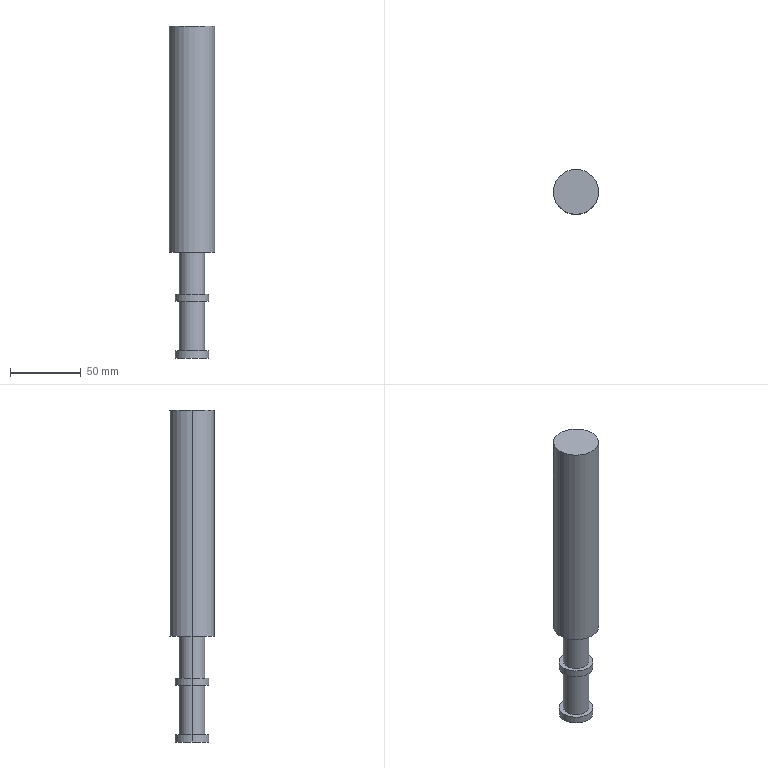Part | SolidWorks | features ICE 4, LPattern 1 | 1 solid | 16 faces | box 32 x 32 x 235 mm | volume 149708 mm3 | cylinder 10 | plane 6 | commonest cylinder face diameters 18 x4 23.904 x4 32 x2
STEP:
#1=CARTESIAN_POINT('',(-28.201,5.869,-90.));
#2=VERTEX_POINT('',#1);
#3=CARTESIAN_POINT('',(-10.201,5.869,-90.));
#4=VERTEX_POINT('',#3);
#5=CARTESIAN_POINT('',(-19.201,5.869,-90.));
#6=DIRECTION('',(0.,0.,-1.));
#7=DIRECTION('',(-1.,0.,0.));
#8=AXIS2_PLACEMENT_3D('',#5,#6,#7);
#9=CIRCLE('',#8,9.);
#10=EDGE_CURVE('',#2,#4,#9,.T.);
#11=ORIENTED_EDGE('',*,*,#10,.F.);
#12=CARTESIAN_POINT('',(-28.201,5.869,-60.));
#13=VERTEX_POINT('',#12);
#14=CARTESIAN_POINT('',(-28.201,5.869,-130.));
#15=DIRECTION('',(0.,0.,1.));
#16=VECTOR('',#15,1000.);
#17=LINE('',#14,#16);
#18=EDGE_CURVE('',#2,#13,#17,.T.);
#19=ORIENTED_EDGE('',*,*,#18,.T.);
#20=CARTESIAN_POINT('',(-10.201,5.869,-60.));
#21=VERTEX_POINT('',#20);
#22=CARTESIAN_POINT('',(-19.201,5.869,-60.));
#23=DIRECTION('',(0.,0.,-1.));
#24=DIRECTION('',(-1.,0.,0.));
#25=AXIS2_PLACEMENT_3D('',#22,#23,#24);
#26=CIRCLE('',#25,9.);
#27=EDGE_CURVE('',#13,#21,#26,.T.);
#28=ORIENTED_EDGE('',*,*,#27,.T.);
#29=CARTESIAN_POINT('',(-10.201,5.869,-130.));
#30=DIRECTION('',(0.,0.,1.));
#31=VECTOR('',#30,1000.);
#32=LINE('',#29,#31);
#33=EDGE_CURVE('',#4,#21,#32,.T.);
#34=ORIENTED_EDGE('',*,*,#33,.F.);
#35=EDGE_LOOP('',(#11,#19,#28,#34));
#36=FACE_OUTER_BOUND('',#35,.T.);
#37=CARTESIAN_POINT('',(-19.201,5.869,-130.));
#38=DIRECTION('',(0.,0.,1.));
#39=DIRECTION('',(1.,0.,0.));
#40=AXIS2_PLACEMENT_3D('',#37,#38,#39);
#41=CYLINDRICAL_SURFACE('',#40,9.);
#42=ADVANCED_FACE('',(#36),#41,.T.);
#43=CARTESIAN_POINT('',(-3.201,5.869,-60.));
#44=VERTEX_POINT('',#43);
#45=CARTESIAN_POINT('',(-35.201,5.869,-60.));
#46=VERTEX_POINT('',#45);
#47=CARTESIAN_POINT('',(-19.201,5.869,-60.));
#48=DIRECTION('',(0.,0.,1.));
#49=DIRECTION('',(1.,0.,0.));
#50=AXIS2_PLACEMENT_3D('',#47,#48,#49);
#51=CIRCLE('',#50,16.);
#52=EDGE_CURVE('',#44,#46,#51,.T.);
#53=ORIENTED_EDGE('',*,*,#52,.T.);
#54=CARTESIAN_POINT('',(-35.201,5.869,100.));
#55=VERTEX_POINT('',#54);
#56=CARTESIAN_POINT('',(-35.201,5.869,-60.));
#57=DIRECTION('',(0.,0.,1.));
#58=VECTOR('',#57,1000.);
#59=LINE('',#56,#58);
#60=EDGE_CURVE('',#46,#55,#59,.T.);
#61=ORIENTED_EDGE('',*,*,#60,.T.);
#62=CARTESIAN_POINT('',(-3.201,5.869,100.));
#63=VERTEX_POINT('',#62);
#64=CARTESIAN_POINT('',(-19.201,5.869,100.));
#65=DIRECTION('',(0.,0.,1.));
#66=DIRECTION('',(1.,0.,0.));
#67=AXIS2_PLACEMENT_3D('',#64,#65,#66);
#68=CIRCLE('',#67,16.);
#69=EDGE_CURVE('',#63,#55,#68,.T.);
#70=ORIENTED_EDGE('',*,*,#69,.F.);
#71=CARTESIAN_POINT('',(-3.201,5.869,-60.));
#72=DIRECTION('',(0.,0.,1.));
#73=VECTOR('',#72,1000.);
#74=LINE('',#71,#73);
#75=EDGE_CURVE('',#44,#63,#74,.T.);
#76=ORIENTED_EDGE('',*,*,#75,.F.);
#77=EDGE_LOOP('',(#53,#61,#70,#76));
#78=FACE_OUTER_BOUND('',#77,.T.);
#79=CARTESIAN_POINT('',(-19.201,5.869,-60.));
#80=DIRECTION('',(0.,0.,1.));
#81=DIRECTION('',(1.,0.,0.));
#82=AXIS2_PLACEMENT_3D('',#79,#80,#81);
#83=CYLINDRICAL_SURFACE('',#82,16.);
#84=ADVANCED_FACE('',(#78),#83,.T.);
#85=CARTESIAN_POINT('',(-31.153,5.869,-95.));
#86=VERTEX_POINT('',#85);
#87=CARTESIAN_POINT('',(-7.249,5.869,-95.));
#88=VERTEX_POINT('',#87);
#89=CARTESIAN_POINT('',(-19.201,5.869,-95.));
#90=DIRECTION('',(0.,0.,-1.));
#91=DIRECTION('',(-1.,0.,0.));
#92=AXIS2_PLACEMENT_3D('',#89,#90,#91);
#93=CIRCLE('',#92,11.952);
#94=EDGE_CURVE('',#86,#88,#93,.T.);
#95=ORIENTED_EDGE('',*,*,#94,.F.);
#96=CARTESIAN_POINT('',(-31.153,5.869,-90.));
#97=VERTEX_POINT('',#96);
#98=CARTESIAN_POINT('',(-31.153,5.869,-95.));
#99=DIRECTION('',(0.,0.,1.));
#100=VECTOR('',#99,1000.);
#101=LINE('',#98,#100);
#102=EDGE_CURVE('',#86,#97,#101,.T.);
#103=ORIENTED_EDGE('',*,*,#102,.T.);
#104=CARTESIAN_POINT('',(-7.249,5.869,-90.));
#105=VERTEX_POINT('',#104);
#106=CARTESIAN_POINT('',(-19.201,5.869,-90.));
#107=DIRECTION('',(0.,0.,-1.));
#108=DIRECTION('',(-1.,0.,0.));
#109=AXIS2_PLACEMENT_3D('',#106,#107,#108);
#110=CIRCLE('',#109,11.952);
#111=EDGE_CURVE('',#97,#105,#110,.T.);
#112=ORIENTED_EDGE('',*,*,#111,.T.);
#113=CARTESIAN_POINT('',(-7.249,5.869,-95.));
#114=DIRECTION('',(0.,0.,1.));
#115=VECTOR('',#114,1000.);
#116=LINE('',#113,#115);
#117=EDGE_CURVE('',#88,#105,#116,.T.);
#118=ORIENTED_EDGE('',*,*,#117,.F.);
#119=EDGE_LOOP('',(#95,#103,#112,#118));
#120=FACE_OUTER_BOUND('',#119,.T.);
#121=CARTESIAN_POINT('',(-19.201,5.869,-95.));
#122=DIRECTION('',(0.,0.,1.));
#123=DIRECTION('',(1.,0.,0.));
#124=AXIS2_PLACEMENT_3D('',#121,#122,#123);
#125=CYLINDRICAL_SURFACE('',#124,11.952);
#126=ADVANCED_FACE('',(#120),#125,.T.);
#127=CARTESIAN_POINT('',(-31.153,5.869,-135.));
#128=VERTEX_POINT('',#127);
#129=CARTESIAN_POINT('',(-7.249,5.869,-135.));
#130=VERTEX_POINT('',#129);
#131=CARTESIAN_POINT('',(-19.201,5.869,-135.));
#132=DIRECTION('',(0.,0.,-1.));
#133=DIRECTION('',(-1.,0.,0.));
#134=AXIS2_PLACEMENT_3D('',#131,#132,#133);
#135=CIRCLE('',#134,11.952);
#136=EDGE_CURVE('',#128,#130,#135,.T.);
#137=ORIENTED_EDGE('',*,*,#136,.F.);
#138=CARTESIAN_POINT('',(-31.153,5.869,-130.));
#139=VERTEX_POINT('',#138);
#140=CARTESIAN_POINT('',(-31.153,5.869,-135.));
#141=DIRECTION('',(0.,0.,1.));
#142=VECTOR('',#141,1000.);
#143=LINE('',#140,#142);
#144=EDGE_CURVE('',#128,#139,#143,.T.);
#145=ORIENTED_EDGE('',*,*,#144,.T.);
#146=CARTESIAN_POINT('',(-7.249,5.869,-130.));
#147=VERTEX_POINT('',#146);
#148=CARTESIAN_POINT('',(-19.201,5.869,-130.));
#149=DIRECTION('',(0.,0.,-1.));
#150=DIRECTION('',(-1.,0.,0.));
#151=AXIS2_PLACEMENT_3D('',#148,#149,#150);
#152=CIRCLE('',#151,11.952);
#153=EDGE_CURVE('',#139,#147,#152,.T.);
#154=ORIENTED_EDGE('',*,*,#153,.T.);
#155=CARTESIAN_POINT('',(-7.249,5.869,-135.));
#156=DIRECTION('',(0.,0.,1.));
#157=VECTOR('',#156,1000.);
#158=LINE('',#155,#157);
#159=EDGE_CURVE('',#130,#147,#158,.T.);
#160=ORIENTED_EDGE('',*,*,#159,.F.);
#161=EDGE_LOOP('',(#137,#145,#154,#160));
#162=FACE_OUTER_BOUND('',#161,.T.);
#163=CARTESIAN_POINT('',(-19.201,5.869,-135.));
#164=DIRECTION('',(0.,0.,1.));
#165=DIRECTION('',(1.,0.,0.));
#166=AXIS2_PLACEMENT_3D('',#163,#164,#165);
#167=CYLINDRICAL_SURFACE('',#166,11.952);
#168=ADVANCED_FACE('',(#162),#167,.T.);
#169=CARTESIAN_POINT('',(-28.201,5.869,-130.));
#170=VERTEX_POINT('',#169);
#171=CARTESIAN_POINT('',(-10.201,5.869,-130.));
#172=VERTEX_POINT('',#171);
#173=CARTESIAN_POINT('',(-19.201,5.869,-130.));
#174=DIRECTION('',(0.,0.,-1.));
#175=DIRECTION('',(-1.,0.,0.));
#176=AXIS2_PLACEMENT_3D('',#173,#174,#175);
#177=CIRCLE('',#176,9.);
#178=EDGE_CURVE('',#170,#172,#177,.T.);
#179=ORIENTED_EDGE('',*,*,#178,.F.);
#180=CARTESIAN_POINT('',(-28.201,5.869,-95.));
#181=VERTEX_POINT('',#180);
#182=CARTESIAN_POINT('',(-28.201,5.869,-130.));
#183=DIRECTION('',(0.,0.,1.));
#184=VECTOR('',#183,1000.);
#185=LINE('',#182,#184);
#186=EDGE_CURVE('',#170,#181,#185,.T.);
#187=ORIENTED_EDGE('',*,*,#186,.T.);
#188=CARTESIAN_POINT('',(-10.201,5.869,-95.));
#189=VERTEX_POINT('',#188);
#190=CARTESIAN_POINT('',(-19.201,5.869,-95.));
#191=DIRECTION('',(0.,0.,-1.));
#192=DIRECTION('',(-1.,0.,0.));
#193=AXIS2_PLACEMENT_3D('',#190,#191,#192);
#194=CIRCLE('',#193,9.);
#195=EDGE_CURVE('',#181,#189,#194,.T.);
#196=ORIENTED_EDGE('',*,*,#195,.T.);
#197=CARTESIAN_POINT('',(-10.201,5.869,-130.));
#198=DIRECTION('',(0.,0.,1.));
#199=VECTOR('',#198,1000.);
#200=LINE('',#197,#199);
#201=EDGE_CURVE('',#172,#189,#200,.T.);
#202=ORIENTED_EDGE('',*,*,#201,.F.);
#203=EDGE_LOOP('',(#179,#187,#196,#202));
#204=FACE_OUTER_BOUND('',#203,.T.);
#205=CARTESIAN_POINT('',(-19.201,5.869,-130.));
#206=DIRECTION('',(0.,0.,1.));
#207=DIRECTION('',(1.,0.,0.));
#208=AXIS2_PLACEMENT_3D('',#205,#206,#207);
#209=CYLINDRICAL_SURFACE('',#208,9.);
#210=ADVANCED_FACE('',(#204),#209,.T.);
#211=ORIENTED_EDGE('',*,*,#186,.F.);
#212=CARTESIAN_POINT('',(-19.201,5.869,-130.));
#213=DIRECTION('',(0.,0.,-1.));
#214=DIRECTION('',(-1.,0.,0.));
#215=AXIS2_PLACEMENT_3D('',#212,#213,#214);
#216=CIRCLE('',#215,9.);
#217=EDGE_CURVE('',#172,#170,#216,.T.);
#218=ORIENTED_EDGE('',*,*,#217,.F.);
#219=ORIENTED_EDGE('',*,*,#201,.T.);
#220=CARTESIAN_POINT('',(-19.201,5.869,-95.));
#221=DIRECTION('',(0.,0.,-1.));
#222=DIRECTION('',(-1.,0.,0.));
#223=AXIS2_PLACEMENT_3D('',#220,#221,#222);
#224=CIRCLE('',#223,9.);
#225=EDGE_CURVE('',#189,#181,#224,.T.);
#226=ORIENTED_EDGE('',*,*,#225,.T.);
#227=EDGE_LOOP('',(#211,#218,#219,#226));
#228=FACE_OUTER_BOUND('',#227,.T.);
#229=CARTESIAN_POINT('',(-19.201,5.869,-130.));
#230=DIRECTION('',(0.,0.,1.));
#231=DIRECTION('',(1.,0.,0.));
#232=AXIS2_PLACEMENT_3D('',#229,#230,#231);
#233=CYLINDRICAL_SURFACE('',#232,9.);
#234=ADVANCED_FACE('',(#228),#233,.T.);
#235=ORIENTED_EDGE('',*,*,#144,.F.);
#236=CARTESIAN_POINT('',(-19.201,5.869,-135.));
#237=DIRECTION('',(0.,0.,-1.));
#238=DIRECTION('',(-1.,0.,0.));
#239=AXIS2_PLACEMENT_3D('',#236,#237,#238);
#240=CIRCLE('',#239,11.952);
#241=EDGE_CURVE('',#130,#128,#240,.T.);
#242=ORIENTED_EDGE('',*,*,#241,.F.);
#243=ORIENTED_EDGE('',*,*,#159,.T.);
#244=CARTESIAN_POINT('',(-19.201,5.869,-130.));
#245=DIRECTION('',(0.,0.,-1.));
#246=DIRECTION('',(-1.,0.,0.));
#247=AXIS2_PLACEMENT_3D('',#244,#245,#246);
#248=CIRCLE('',#247,11.952);
#249=EDGE_CURVE('',#147,#139,#248,.T.);
#250=ORIENTED_EDGE('',*,*,#249,.T.);
#251=EDGE_LOOP('',(#235,#242,#243,#250));
#252=FACE_OUTER_BOUND('',#251,.T.);
#253=CARTESIAN_POINT('',(-19.201,5.869,-135.));
#254=DIRECTION('',(0.,0.,1.));
#255=DIRECTION('',(1.,0.,0.));
#256=AXIS2_PLACEMENT_3D('',#253,#254,#255);
#257=CYLINDRICAL_SURFACE('',#256,11.952);
#258=ADVANCED_FACE('',(#252),#257,.T.);
#259=ORIENTED_EDGE('',*,*,#241,.T.);
#260=ORIENTED_EDGE('',*,*,#136,.T.);
#261=EDGE_LOOP('',(#259,#260));
#262=FACE_OUTER_BOUND('',#261,.T.);
#263=CARTESIAN_POINT('',(-19.201,5.869,-135.));
#264=DIRECTION('',(0.,0.,-1.));
#265=DIRECTION('',(-1.,0.,0.));
#266=AXIS2_PLACEMENT_3D('',#263,#264,#265);
#267=PLANE('',#266);
#268=ADVANCED_FACE('',(#262),#267,.T.);
#269=ORIENTED_EDGE('',*,*,#217,.T.);
#270=ORIENTED_EDGE('',*,*,#178,.T.);
#271=EDGE_LOOP('',(#269,#270));
#272=FACE_BOUND('',#271,.T.);
#273=ORIENTED_EDGE('',*,*,#249,.F.);
#274=ORIENTED_EDGE('',*,*,#153,.F.);
#275=EDGE_LOOP('',(#273,#274));
#276=FACE_OUTER_BOUND('',#275,.T.);
#277=CARTESIAN_POINT('',(-19.201,5.869,-130.));
#278=DIRECTION('',(0.,0.,-1.));
#279=DIRECTION('',(-1.,0.,0.));
#280=AXIS2_PLACEMENT_3D('',#277,#278,#279);
#281=PLANE('',#280);
#282=ADVANCED_FACE('',(#272,#276),#281,.F.);
#283=ORIENTED_EDGE('',*,*,#102,.F.);
#284=CARTESIAN_POINT('',(-19.201,5.869,-95.));
#285=DIRECTION('',(0.,0.,-1.));
#286=DIRECTION('',(-1.,0.,0.));
#287=AXIS2_PLACEMENT_3D('',#284,#285,#286);
#288=CIRCLE('',#287,11.952);
#289=EDGE_CURVE('',#88,#86,#288,.T.);
#290=ORIENTED_EDGE('',*,*,#289,.F.);
#291=ORIENTED_EDGE('',*,*,#117,.T.);
#292=CARTESIAN_POINT('',(-19.201,5.869,-90.));
#293=DIRECTION('',(0.,0.,-1.));
#294=DIRECTION('',(-1.,0.,0.));
#295=AXIS2_PLACEMENT_3D('',#292,#293,#294);
#296=CIRCLE('',#295,11.952);
#297=EDGE_CURVE('',#105,#97,#296,.T.);
#298=ORIENTED_EDGE('',*,*,#297,.T.);
#299=EDGE_LOOP('',(#283,#290,#291,#298));
#300=FACE_OUTER_BOUND('',#299,.T.);
#301=CARTESIAN_POINT('',(-19.201,5.869,-95.));
#302=DIRECTION('',(0.,0.,1.));
#303=DIRECTION('',(1.,0.,0.));
#304=AXIS2_PLACEMENT_3D('',#301,#302,#303);
#305=CYLINDRICAL_SURFACE('',#304,11.952);
#306=ADVANCED_FACE('',(#300),#305,.T.);
#307=ORIENTED_EDGE('',*,*,#225,.F.);
#308=ORIENTED_EDGE('',*,*,#195,.F.);
#309=EDGE_LOOP('',(#307,#308));
#310=FACE_BOUND('',#309,.T.);
#311=ORIENTED_EDGE('',*,*,#289,.T.);
#312=ORIENTED_EDGE('',*,*,#94,.T.);
#313=EDGE_LOOP('',(#311,#312));
#314=FACE_OUTER_BOUND('',#313,.T.);
#315=CARTESIAN_POINT('',(-19.201,5.869,-95.));
#316=DIRECTION('',(0.,0.,-1.));
#317=DIRECTION('',(-1.,0.,0.));
#318=AXIS2_PLACEMENT_3D('',#315,#316,#317);
#319=PLANE('',#318);
#320=ADVANCED_FACE('',(#310,#314),#319,.T.);
#321=CARTESIAN_POINT('',(-19.201,5.869,-90.));
#322=DIRECTION('',(0.,0.,-1.));
#323=DIRECTION('',(-1.,0.,0.));
#324=AXIS2_PLACEMENT_3D('',#321,#322,#323);
#325=CIRCLE('',#324,9.);
#326=EDGE_CURVE('',#4,#2,#325,.T.);
#327=ORIENTED_EDGE('',*,*,#326,.T.);
#328=ORIENTED_EDGE('',*,*,#10,.T.);
#329=EDGE_LOOP('',(#327,#328));
#330=FACE_BOUND('',#329,.T.);
#331=ORIENTED_EDGE('',*,*,#297,.F.);
#332=ORIENTED_EDGE('',*,*,#111,.F.);
#333=EDGE_LOOP('',(#331,#332));
#334=FACE_OUTER_BOUND('',#333,.T.);
#335=CARTESIAN_POINT('',(-19.201,5.869,-90.));
#336=DIRECTION('',(0.,0.,-1.));
#337=DIRECTION('',(-1.,0.,0.));
#338=AXIS2_PLACEMENT_3D('',#335,#336,#337);
#339=PLANE('',#338);
#340=ADVANCED_FACE('',(#330,#334),#339,.F.);
#341=ORIENTED_EDGE('',*,*,#69,.T.);
#342=CARTESIAN_POINT('',(-19.201,5.869,100.));
#343=DIRECTION('',(0.,0.,1.));
#344=DIRECTION('',(1.,0.,0.));
#345=AXIS2_PLACEMENT_3D('',#342,#343,#344);
#346=CIRCLE('',#345,16.);
#347=EDGE_CURVE('',#55,#63,#346,.T.);
#348=ORIENTED_EDGE('',*,*,#347,.T.);
#349=EDGE_LOOP('',(#341,#348));
#350=FACE_OUTER_BOUND('',#349,.T.);
#351=CARTESIAN_POINT('',(-19.201,5.869,100.));
#352=DIRECTION('',(0.,0.,1.));
#353=DIRECTION('',(1.,0.,0.));
#354=AXIS2_PLACEMENT_3D('',#351,#352,#353);
#355=PLANE('',#354);
#356=ADVANCED_FACE('',(#350),#355,.T.);
#357=ORIENTED_EDGE('',*,*,#60,.F.);
#358=CARTESIAN_POINT('',(-19.201,5.869,-60.));
#359=DIRECTION('',(0.,0.,1.));
#360=DIRECTION('',(1.,0.,0.));
#361=AXIS2_PLACEMENT_3D('',#358,#359,#360);
#362=CIRCLE('',#361,16.);
#363=EDGE_CURVE('',#46,#44,#362,.T.);
#364=ORIENTED_EDGE('',*,*,#363,.T.);
#365=ORIENTED_EDGE('',*,*,#75,.T.);
#366=ORIENTED_EDGE('',*,*,#347,.F.);
#367=EDGE_LOOP('',(#357,#364,#365,#366));
#368=FACE_OUTER_BOUND('',#367,.T.);
#369=CARTESIAN_POINT('',(-19.201,5.869,-60.));
#370=DIRECTION('',(0.,0.,1.));
#371=DIRECTION('',(1.,0.,0.));
#372=AXIS2_PLACEMENT_3D('',#369,#370,#371);
#373=CYLINDRICAL_SURFACE('',#372,16.);
#374=ADVANCED_FACE('',(#368),#373,.T.);
#375=CARTESIAN_POINT('',(-19.201,5.869,-60.));
#376=DIRECTION('',(0.,0.,-1.));
#377=DIRECTION('',(-1.,0.,0.));
#378=AXIS2_PLACEMENT_3D('',#375,#376,#377);
#379=CIRCLE('',#378,9.);
#380=EDGE_CURVE('',#21,#13,#379,.T.);
#381=ORIENTED_EDGE('',*,*,#380,.F.);
#382=ORIENTED_EDGE('',*,*,#27,.F.);
#383=EDGE_LOOP('',(#381,#382));
#384=FACE_BOUND('',#383,.T.);
#385=ORIENTED_EDGE('',*,*,#52,.F.);
#386=ORIENTED_EDGE('',*,*,#363,.F.);
#387=EDGE_LOOP('',(#385,#386));
#388=FACE_OUTER_BOUND('',#387,.T.);
#389=CARTESIAN_POINT('',(-19.201,5.869,-60.));
#390=DIRECTION('',(0.,0.,1.));
#391=DIRECTION('',(1.,0.,0.));
#392=AXIS2_PLACEMENT_3D('',#389,#390,#391);
#393=PLANE('',#392);
#394=ADVANCED_FACE('',(#384,#388),#393,.F.);
#395=ORIENTED_EDGE('',*,*,#18,.F.);
#396=ORIENTED_EDGE('',*,*,#326,.F.);
#397=ORIENTED_EDGE('',*,*,#33,.T.);
#398=ORIENTED_EDGE('',*,*,#380,.T.);
#399=EDGE_LOOP('',(#395,#396,#397,#398));
#400=FACE_OUTER_BOUND('',#399,.T.);
#401=CARTESIAN_POINT('',(-19.201,5.869,-130.));
#402=DIRECTION('',(0.,0.,1.));
#403=DIRECTION('',(1.,0.,0.));
#404=AXIS2_PLACEMENT_3D('',#401,#402,#403);
#405=CYLINDRICAL_SURFACE('',#404,9.);
#406=ADVANCED_FACE('',(#400),#405,.T.);
#407=CLOSED_SHELL('',(#42,#84,#126,#168,#210,#234,#258,#268,#282,#306,#320,#340,#356,#374,#394,#406));
#408=MANIFOLD_SOLID_BREP('',#407);
#409=CARTESIAN_POINT('',(0.,0.,0.));
#410=DIRECTION('',(0.,0.,1.));
#411=DIRECTION('',(1.,0.,0.));
#412=AXIS2_PLACEMENT_3D('',#409,#410,#411);
#413=(LENGTH_UNIT()NAMED_UNIT(*)SI_UNIT(.MILLI.,.METRE.));
#414=UNCERTAINTY_MEASURE_WITH_UNIT(LENGTH_MEASURE(0.00001),#413,'','');
#415=(NAMED_UNIT(*)PLANE_ANGLE_UNIT()SI_UNIT($,.RADIAN.));
#416=(NAMED_UNIT(*)SI_UNIT($,.STERADIAN.)SOLID_ANGLE_UNIT());
#417=(GEOMETRIC_REPRESENTATION_CONTEXT(3)GLOBAL_UNCERTAINTY_ASSIGNED_CONTEXT((#414))GLOBAL_UNIT_ASSIGNED_CONTEXT((#413,#415,#416))REPRESENTATION_CONTEXT('',''));
#418=ADVANCED_BREP_SHAPE_REPRESENTATION('',(#408,#412),#417);